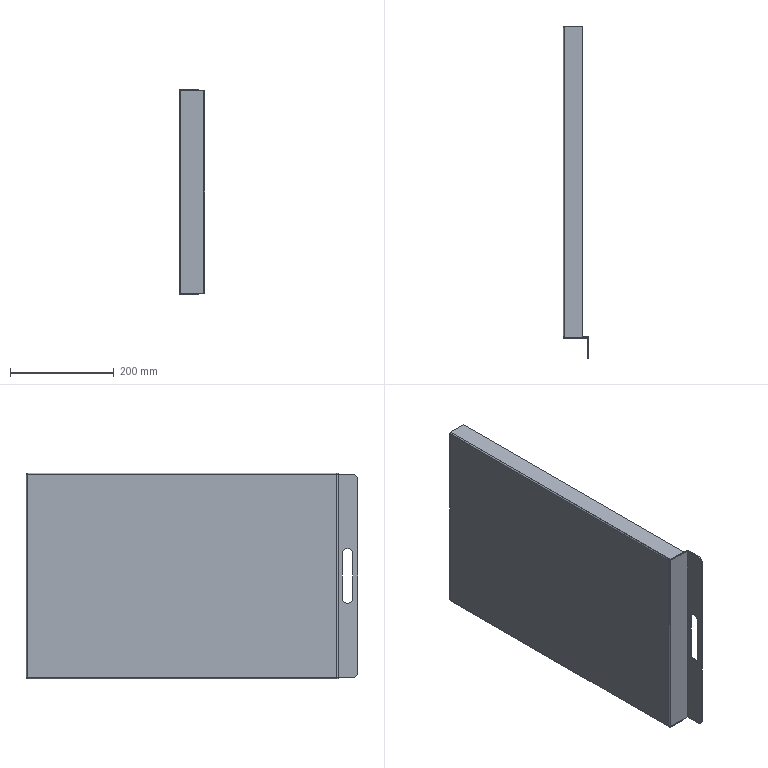Part | STEP file | HJDX-306 | 1 solid | 49 faces | box 50 x 638 x 396 mm | volume 649767 mm3 | plane 34 | cylinder 15 | commonest cylinder face diameters 1 x5 5 x5 20 x5
STEP:
#1=CARTESIAN_POINT('',(46.,-318.,-52.752));
#2=VERTEX_POINT('',#1);
#3=CARTESIAN_POINT('',(46.,-308.,-42.752));
#4=VERTEX_POINT('',#3);
#5=CARTESIAN_POINT('',(46.,-318.,-42.752));
#6=DIRECTION('',(1.,0.,0.));
#7=DIRECTION('',(0.,0.,-1.));
#8=AXIS2_PLACEMENT_3D('',#5,#6,#7);
#9=CIRCLE('',#8,10.);
#10=EDGE_CURVE('',#2,#4,#9,.T.);
#11=ORIENTED_EDGE('',*,*,#10,.F.);
#12=CARTESIAN_POINT('',(48.,-318.,-52.752));
#13=VERTEX_POINT('',#12);
#14=CARTESIAN_POINT('',(-2.,-318.,-52.752));
#15=DIRECTION('',(1.,0.,0.));
#16=VECTOR('',#15,1000.);
#17=LINE('',#14,#16);
#18=EDGE_CURVE('',#2,#13,#17,.T.);
#19=ORIENTED_EDGE('',*,*,#18,.T.);
#20=CARTESIAN_POINT('',(48.,-308.,-42.752));
#21=VERTEX_POINT('',#20);
#22=CARTESIAN_POINT('',(48.,-318.,-42.752));
#23=DIRECTION('',(-1.,0.,0.));
#24=DIRECTION('',(0.,0.,-1.));
#25=AXIS2_PLACEMENT_3D('',#22,#23,#24);
#26=CIRCLE('',#25,10.);
#27=EDGE_CURVE('',#21,#13,#26,.T.);
#28=ORIENTED_EDGE('',*,*,#27,.F.);
#29=CARTESIAN_POINT('',(-2.,-308.,-42.752));
#30=DIRECTION('',(-1.,0.,0.));
#31=VECTOR('',#30,1000.);
#32=LINE('',#29,#31);
#33=EDGE_CURVE('',#21,#4,#32,.T.);
#34=ORIENTED_EDGE('',*,*,#33,.T.);
#35=EDGE_LOOP('',(#11,#19,#28,#34));
#36=FACE_OUTER_BOUND('',#35,.T.);
#37=CARTESIAN_POINT('',(-2.,-318.,-42.752));
#38=DIRECTION('',(1.,0.,0.));
#39=DIRECTION('',(0.,0.,-1.));
#40=AXIS2_PLACEMENT_3D('',#37,#38,#39);
#41=CYLINDRICAL_SURFACE('',#40,10.);
#42=ADVANCED_FACE('',(#36),#41,.F.);
#43=CARTESIAN_POINT('',(-2.,-297.5,195.5));
#44=VERTEX_POINT('',#43);
#45=CARTESIAN_POINT('',(-2.,297.5,195.5));
#46=VERTEX_POINT('',#45);
#47=CARTESIAN_POINT('',(-2.,0.,195.5));
#48=DIRECTION('',(0.,1.,0.));
#49=VECTOR('',#48,1000.);
#50=LINE('',#47,#49);
#51=EDGE_CURVE('',#44,#46,#50,.T.);
#52=ORIENTED_EDGE('',*,*,#51,.T.);
#53=CARTESIAN_POINT('',(-2.,297.5,-195.5));
#54=VERTEX_POINT('',#53);
#55=CARTESIAN_POINT('',(-2.,297.5,0.));
#56=DIRECTION('',(0.,0.,-1.));
#57=VECTOR('',#56,1000.);
#58=LINE('',#55,#57);
#59=EDGE_CURVE('',#46,#54,#58,.T.);
#60=ORIENTED_EDGE('',*,*,#59,.T.);
#61=CARTESIAN_POINT('',(-2.,-297.5,-195.5));
#62=VERTEX_POINT('',#61);
#63=CARTESIAN_POINT('',(-2.,0.,-195.5));
#64=DIRECTION('',(0.,-1.,0.));
#65=VECTOR('',#64,1000.);
#66=LINE('',#63,#65);
#67=EDGE_CURVE('',#54,#62,#66,.T.);
#68=ORIENTED_EDGE('',*,*,#67,.T.);
#69=CARTESIAN_POINT('',(-2.,-297.5,0.));
#70=DIRECTION('',(0.,0.,1.));
#71=VECTOR('',#70,1000.);
#72=LINE('',#69,#71);
#73=EDGE_CURVE('',#62,#44,#72,.T.);
#74=ORIENTED_EDGE('',*,*,#73,.T.);
#75=EDGE_LOOP('',(#52,#60,#68,#74));
#76=FACE_OUTER_BOUND('',#75,.T.);
#77=CARTESIAN_POINT('',(-2.,0.,0.));
#78=DIRECTION('',(-1.,0.,0.));
#79=DIRECTION('',(0.,0.,1.));
#80=AXIS2_PLACEMENT_3D('',#77,#78,#79);
#81=PLANE('',#80);
#82=ADVANCED_FACE('',(#76),#81,.T.);
#83=CARTESIAN_POINT('',(0.5,300.,195.5));
#84=VERTEX_POINT('',#83);
#85=CARTESIAN_POINT('',(0.5,300.,-195.5));
#86=VERTEX_POINT('',#85);
#87=CARTESIAN_POINT('',(0.5,300.,195.5));
#88=DIRECTION('',(0.,0.,-1.));
#89=VECTOR('',#88,1000.);
#90=LINE('',#87,#89);
#91=EDGE_CURVE('',#84,#86,#90,.T.);
#92=ORIENTED_EDGE('',*,*,#91,.T.);
#93=CARTESIAN_POINT('',(0.5,297.5,-195.5));
#94=DIRECTION('',(0.,0.,1.));
#95=DIRECTION('',(1.,0.,0.));
#96=AXIS2_PLACEMENT_3D('',#93,#94,#95);
#97=CIRCLE('',#96,2.5);
#98=EDGE_CURVE('',#86,#54,#97,.T.);
#99=ORIENTED_EDGE('',*,*,#98,.T.);
#100=ORIENTED_EDGE('',*,*,#59,.F.);
#101=CARTESIAN_POINT('',(0.5,297.5,195.5));
#102=DIRECTION('',(0.,0.,-1.));
#103=DIRECTION('',(1.,0.,0.));
#104=AXIS2_PLACEMENT_3D('',#101,#102,#103);
#105=CIRCLE('',#104,2.5);
#106=EDGE_CURVE('',#46,#84,#105,.T.);
#107=ORIENTED_EDGE('',*,*,#106,.T.);
#108=EDGE_LOOP('',(#92,#99,#100,#107));
#109=FACE_OUTER_BOUND('',#108,.T.);
#110=CARTESIAN_POINT('',(0.5,297.5,195.5));
#111=DIRECTION('',(0.,0.,1.));
#112=DIRECTION('',(1.,0.,0.));
#113=AXIS2_PLACEMENT_3D('',#110,#111,#112);
#114=CYLINDRICAL_SURFACE('',#113,2.5);
#115=ADVANCED_FACE('',(#109),#114,.T.);
#116=CARTESIAN_POINT('',(0.5,-297.5,198.));
#117=VERTEX_POINT('',#116);
#118=CARTESIAN_POINT('',(0.5,297.5,198.));
#119=VERTEX_POINT('',#118);
#120=CARTESIAN_POINT('',(0.5,-300.,198.));
#121=DIRECTION('',(0.,1.,0.));
#122=VECTOR('',#121,1000.);
#123=LINE('',#120,#122);
#124=EDGE_CURVE('',#117,#119,#123,.T.);
#125=ORIENTED_EDGE('',*,*,#124,.T.);
#126=CARTESIAN_POINT('',(0.5,297.5,195.5));
#127=DIRECTION('',(0.,-1.,0.));
#128=DIRECTION('',(0.,0.,-1.));
#129=AXIS2_PLACEMENT_3D('',#126,#127,#128);
#130=CIRCLE('',#129,2.5);
#131=EDGE_CURVE('',#119,#46,#130,.T.);
#132=ORIENTED_EDGE('',*,*,#131,.T.);
#133=ORIENTED_EDGE('',*,*,#51,.F.);
#134=CARTESIAN_POINT('',(0.5,-297.5,195.5));
#135=DIRECTION('',(0.,1.,0.));
#136=DIRECTION('',(0.,0.,-1.));
#137=AXIS2_PLACEMENT_3D('',#134,#135,#136);
#138=CIRCLE('',#137,2.5);
#139=EDGE_CURVE('',#44,#117,#138,.T.);
#140=ORIENTED_EDGE('',*,*,#139,.T.);
#141=EDGE_LOOP('',(#125,#132,#133,#140));
#142=FACE_OUTER_BOUND('',#141,.T.);
#143=CARTESIAN_POINT('',(0.5,-300.,195.5));
#144=DIRECTION('',(0.,-1.,0.));
#145=DIRECTION('',(0.,0.,-1.));
#146=AXIS2_PLACEMENT_3D('',#143,#144,#145);
#147=CYLINDRICAL_SURFACE('',#146,2.5);
#148=ADVANCED_FACE('',(#142),#147,.T.);
#149=CARTESIAN_POINT('',(0.5,-300.,-195.5));
#150=VERTEX_POINT('',#149);
#151=CARTESIAN_POINT('',(0.5,-300.,195.5));
#152=VERTEX_POINT('',#151);
#153=CARTESIAN_POINT('',(0.5,-300.,-195.5));
#154=DIRECTION('',(0.,0.,1.));
#155=VECTOR('',#154,1000.);
#156=LINE('',#153,#155);
#157=EDGE_CURVE('',#150,#152,#156,.T.);
#158=ORIENTED_EDGE('',*,*,#157,.T.);
#159=CARTESIAN_POINT('',(0.5,-297.5,195.5));
#160=DIRECTION('',(0.,0.,-1.));
#161=DIRECTION('',(-1.,0.,0.));
#162=AXIS2_PLACEMENT_3D('',#159,#160,#161);
#163=CIRCLE('',#162,2.5);
#164=EDGE_CURVE('',#152,#44,#163,.T.);
#165=ORIENTED_EDGE('',*,*,#164,.T.);
#166=ORIENTED_EDGE('',*,*,#73,.F.);
#167=CARTESIAN_POINT('',(0.5,-297.5,-195.5));
#168=DIRECTION('',(0.,0.,1.));
#169=DIRECTION('',(-1.,0.,0.));
#170=AXIS2_PLACEMENT_3D('',#167,#168,#169);
#171=CIRCLE('',#170,2.5);
#172=EDGE_CURVE('',#62,#150,#171,.T.);
#173=ORIENTED_EDGE('',*,*,#172,.T.);
#174=EDGE_LOOP('',(#158,#165,#166,#173));
#175=FACE_OUTER_BOUND('',#174,.T.);
#176=CARTESIAN_POINT('',(0.5,-297.5,-195.5));
#177=DIRECTION('',(0.,0.,-1.));
#178=DIRECTION('',(-1.,0.,0.));
#179=AXIS2_PLACEMENT_3D('',#176,#177,#178);
#180=CYLINDRICAL_SURFACE('',#179,2.5);
#181=ADVANCED_FACE('',(#175),#180,.T.);
#182=ORIENTED_EDGE('',*,*,#67,.F.);
#183=CARTESIAN_POINT('',(0.5,297.5,-198.));
#184=VERTEX_POINT('',#183);
#185=CARTESIAN_POINT('',(0.5,297.5,-195.5));
#186=DIRECTION('',(0.,-1.,0.));
#187=DIRECTION('',(0.,0.,1.));
#188=AXIS2_PLACEMENT_3D('',#185,#186,#187);
#189=CIRCLE('',#188,2.5);
#190=EDGE_CURVE('',#54,#184,#189,.T.);
#191=ORIENTED_EDGE('',*,*,#190,.T.);
#192=CARTESIAN_POINT('',(0.5,-297.5,-198.));
#193=VERTEX_POINT('',#192);
#194=CARTESIAN_POINT('',(0.5,300.,-198.));
#195=DIRECTION('',(0.,-1.,0.));
#196=VECTOR('',#195,1000.);
#197=LINE('',#194,#196);
#198=EDGE_CURVE('',#184,#193,#197,.T.);
#199=ORIENTED_EDGE('',*,*,#198,.T.);
#200=CARTESIAN_POINT('',(0.5,-297.5,-195.5));
#201=DIRECTION('',(0.,1.,0.));
#202=DIRECTION('',(0.,0.,1.));
#203=AXIS2_PLACEMENT_3D('',#200,#201,#202);
#204=CIRCLE('',#203,2.5);
#205=EDGE_CURVE('',#193,#62,#204,.T.);
#206=ORIENTED_EDGE('',*,*,#205,.T.);
#207=EDGE_LOOP('',(#182,#191,#199,#206));
#208=FACE_OUTER_BOUND('',#207,.T.);
#209=CARTESIAN_POINT('',(0.5,300.,-195.5));
#210=DIRECTION('',(0.,1.,0.));
#211=DIRECTION('',(0.,0.,1.));
#212=AXIS2_PLACEMENT_3D('',#209,#210,#211);
#213=CYLINDRICAL_SURFACE('',#212,2.5);
#214=ADVANCED_FACE('',(#208),#213,.T.);
#215=CARTESIAN_POINT('',(0.,297.5,-195.5));
#216=VERTEX_POINT('',#215);
#217=CARTESIAN_POINT('',(0.5,297.5,-195.5));
#218=DIRECTION('',(-1.,0.,0.));
#219=VECTOR('',#218,1000.);
#220=LINE('',#217,#219);
#221=EDGE_CURVE('',#216,#54,#220,.T.);
#222=ORIENTED_EDGE('',*,*,#221,.T.);
#223=ORIENTED_EDGE('',*,*,#98,.F.);
#224=CARTESIAN_POINT('',(36.,300.,-195.5));
#225=VERTEX_POINT('',#224);
#226=CARTESIAN_POINT('',(0.,300.,-195.5));
#227=DIRECTION('',(1.,0.,0.));
#228=VECTOR('',#227,1000.);
#229=LINE('',#226,#228);
#230=EDGE_CURVE('',#86,#225,#229,.T.);
#231=ORIENTED_EDGE('',*,*,#230,.T.);
#232=CARTESIAN_POINT('',(36.,298.,-195.5));
#233=VERTEX_POINT('',#232);
#234=CARTESIAN_POINT('',(36.,300.,-195.5));
#235=DIRECTION('',(0.,1.,0.));
#236=VECTOR('',#235,1000.);
#237=LINE('',#234,#236);
#238=EDGE_CURVE('',#233,#225,#237,.T.);
#239=ORIENTED_EDGE('',*,*,#238,.F.);
#240=CARTESIAN_POINT('',(0.5,298.,-195.5));
#241=VERTEX_POINT('',#240);
#242=CARTESIAN_POINT('',(0.,298.,-195.5));
#243=DIRECTION('',(1.,0.,0.));
#244=VECTOR('',#243,1000.);
#245=LINE('',#242,#244);
#246=EDGE_CURVE('',#241,#233,#245,.T.);
#247=ORIENTED_EDGE('',*,*,#246,.F.);
#248=CARTESIAN_POINT('',(0.5,297.5,-195.5));
#249=DIRECTION('',(0.,0.,1.));
#250=DIRECTION('',(1.,0.,0.));
#251=AXIS2_PLACEMENT_3D('',#248,#249,#250);
#252=CIRCLE('',#251,0.5);
#253=EDGE_CURVE('',#241,#216,#252,.T.);
#254=ORIENTED_EDGE('',*,*,#253,.T.);
#255=EDGE_LOOP('',(#222,#223,#231,#239,#247,#254));
#256=FACE_OUTER_BOUND('',#255,.T.);
#257=CARTESIAN_POINT('',(0.5,297.5,-195.5));
#258=DIRECTION('',(0.,0.,-1.));
#259=DIRECTION('',(-1.,0.,0.));
#260=AXIS2_PLACEMENT_3D('',#257,#258,#259);
#261=PLANE('',#260);
#262=ADVANCED_FACE('',(#256),#261,.T.);
#263=CARTESIAN_POINT('',(36.,300.,195.5));
#264=VERTEX_POINT('',#263);
#265=CARTESIAN_POINT('',(0.,300.,195.5));
#266=DIRECTION('',(-1.,0.,0.));
#267=VECTOR('',#266,1000.);
#268=LINE('',#265,#267);
#269=EDGE_CURVE('',#264,#84,#268,.T.);
#270=ORIENTED_EDGE('',*,*,#269,.F.);
#271=CARTESIAN_POINT('',(36.,300.,0.));
#272=DIRECTION('',(0.,0.,1.));
#273=VECTOR('',#272,1000.);
#274=LINE('',#271,#273);
#275=EDGE_CURVE('',#225,#264,#274,.T.);
#276=ORIENTED_EDGE('',*,*,#275,.F.);
#277=ORIENTED_EDGE('',*,*,#230,.F.);
#278=ORIENTED_EDGE('',*,*,#91,.F.);
#279=EDGE_LOOP('',(#270,#276,#277,#278));
#280=FACE_OUTER_BOUND('',#279,.T.);
#281=CARTESIAN_POINT('',(0.,300.,0.));
#282=DIRECTION('',(0.,-1.,0.));
#283=DIRECTION('',(1.,0.,0.));
#284=AXIS2_PLACEMENT_3D('',#281,#282,#283);
#285=PLANE('',#284);
#286=ADVANCED_FACE('',(#280),#285,.F.);
#287=CARTESIAN_POINT('',(0.,297.5,195.5));
#288=VERTEX_POINT('',#287);
#289=CARTESIAN_POINT('',(0.5,298.,195.5));
#290=VERTEX_POINT('',#289);
#291=CARTESIAN_POINT('',(0.5,297.5,195.5));
#292=DIRECTION('',(0.,0.,-1.));
#293=DIRECTION('',(1.,0.,0.));
#294=AXIS2_PLACEMENT_3D('',#291,#292,#293);
#295=CIRCLE('',#294,0.5);
#296=EDGE_CURVE('',#288,#290,#295,.T.);
#297=ORIENTED_EDGE('',*,*,#296,.T.);
#298=CARTESIAN_POINT('',(36.,298.,195.5));
#299=VERTEX_POINT('',#298);
#300=CARTESIAN_POINT('',(36.,298.,195.5));
#301=DIRECTION('',(-1.,0.,0.));
#302=VECTOR('',#301,1000.);
#303=LINE('',#300,#302);
#304=EDGE_CURVE('',#299,#290,#303,.T.);
#305=ORIENTED_EDGE('',*,*,#304,.F.);
#306=CARTESIAN_POINT('',(36.,300.,195.5));
#307=DIRECTION('',(0.,-1.,0.));
#308=VECTOR('',#307,1000.);
#309=LINE('',#306,#308);
#310=EDGE_CURVE('',#264,#299,#309,.T.);
#311=ORIENTED_EDGE('',*,*,#310,.F.);
#312=ORIENTED_EDGE('',*,*,#269,.T.);
#313=ORIENTED_EDGE('',*,*,#106,.F.);
#314=CARTESIAN_POINT('',(0.5,297.5,195.5));
#315=DIRECTION('',(-1.,0.,0.));
#316=VECTOR('',#315,1000.);
#317=LINE('',#314,#316);
#318=EDGE_CURVE('',#288,#46,#317,.T.);
#319=ORIENTED_EDGE('',*,*,#318,.F.);
#320=EDGE_LOOP('',(#297,#305,#311,#312,#313,#319));
#321=FACE_OUTER_BOUND('',#320,.T.);
#322=CARTESIAN_POINT('',(0.5,297.5,195.5));
#323=DIRECTION('',(0.,0.,-1.));
#324=DIRECTION('',(-1.,0.,0.));
#325=AXIS2_PLACEMENT_3D('',#322,#323,#324);
#326=PLANE('',#325);
#327=ADVANCED_FACE('',(#321),#326,.F.);
#328=CARTESIAN_POINT('',(0.5,297.5,196.));
#329=VERTEX_POINT('',#328);
#330=CARTESIAN_POINT('',(0.5,297.5,195.5));
#331=DIRECTION('',(0.,-1.,0.));
#332=DIRECTION('',(0.,0.,-1.));
#333=AXIS2_PLACEMENT_3D('',#330,#331,#332);
#334=CIRCLE('',#333,0.5);
#335=EDGE_CURVE('',#329,#288,#334,.T.);
#336=ORIENTED_EDGE('',*,*,#335,.T.);
#337=ORIENTED_EDGE('',*,*,#318,.T.);
#338=ORIENTED_EDGE('',*,*,#131,.F.);
#339=CARTESIAN_POINT('',(0.5,297.5,195.5));
#340=DIRECTION('',(0.,0.,-1.));
#341=VECTOR('',#340,1000.);
#342=LINE('',#339,#341);
#343=EDGE_CURVE('',#119,#329,#342,.T.);
#344=ORIENTED_EDGE('',*,*,#343,.T.);
#345=EDGE_LOOP('',(#336,#337,#338,#344));
#346=FACE_OUTER_BOUND('',#345,.T.);
#347=CARTESIAN_POINT('',(0.5,297.5,195.5));
#348=DIRECTION('',(0.,1.,0.));
#349=DIRECTION('',(0.,0.,1.));
#350=AXIS2_PLACEMENT_3D('',#347,#348,#349);
#351=PLANE('',#350);
#352=ADVANCED_FACE('',(#346),#351,.T.);
#353=CARTESIAN_POINT('',(36.,-300.,198.));
#354=VERTEX_POINT('',#353);
#355=CARTESIAN_POINT('',(0.5,-300.,198.));
#356=VERTEX_POINT('',#355);
#357=CARTESIAN_POINT('',(0.,-300.,198.));
#358=DIRECTION('',(-1.,0.,0.));
#359=VECTOR('',#358,1000.);
#360=LINE('',#357,#359);
#361=EDGE_CURVE('',#354,#356,#360,.T.);
#362=ORIENTED_EDGE('',*,*,#361,.F.);
#363=CARTESIAN_POINT('',(36.,300.,198.));
#364=VERTEX_POINT('',#363);
#365=CARTESIAN_POINT('',(36.,0.,198.));
#366=DIRECTION('',(0.,-1.,0.));
#367=VECTOR('',#366,1000.);
#368=LINE('',#365,#367);
#369=EDGE_CURVE('',#364,#354,#368,.T.);
#370=ORIENTED_EDGE('',*,*,#369,.F.);
#371=CARTESIAN_POINT('',(0.5,300.,198.));
#372=VERTEX_POINT('',#371);
#373=CARTESIAN_POINT('',(0.,300.,198.));
#374=DIRECTION('',(1.,0.,0.));
#375=VECTOR('',#374,1000.);
#376=LINE('',#373,#375);
#377=EDGE_CURVE('',#372,#364,#376,.T.);
#378=ORIENTED_EDGE('',*,*,#377,.F.);
#379=CARTESIAN_POINT('',(0.5,0.,198.));
#380=DIRECTION('',(0.,1.,0.));
#381=VECTOR('',#380,1000.);
#382=LINE('',#379,#381);
#383=EDGE_CURVE('',#119,#372,#382,.T.);
#384=ORIENTED_EDGE('',*,*,#383,.F.);
#385=ORIENTED_EDGE('',*,*,#124,.F.);
#386=CARTESIAN_POINT('',(0.5,0.,198.));
#387=DIRECTION('',(0.,1.,0.));
#388=VECTOR('',#387,1000.);
#389=LINE('',#386,#388);
#390=EDGE_CURVE('',#356,#117,#389,.T.);
#391=ORIENTED_EDGE('',*,*,#390,.F.);
#392=EDGE_LOOP('',(#362,#370,#378,#384,#385,#391));
#393=FACE_OUTER_BOUND('',#392,.T.);
#394=CARTESIAN_POINT('',(0.,0.,198.));
#395=DIRECTION('',(0.,0.,-1.));
#396=DIRECTION('',(-1.,0.,0.));
#397=AXIS2_PLACEMENT_3D('',#394,#395,#396);
#398=PLANE('',#397);
#399=ADVANCED_FACE('',(#393),#398,.F.);
#400=ORIENTED_EDGE('',*,*,#139,.F.);
#401=CARTESIAN_POINT('',(0.,-297.5,195.5));
#402=VERTEX_POINT('',#401);
#403=CARTESIAN_POINT('',(0.5,-297.5,195.5));
#404=DIRECTION('',(1.,0.,0.));
#405=VECTOR('',#404,1000.);
#406=LINE('',#403,#405);
#407=EDGE_CURVE('',#44,#402,#406,.T.);
#408=ORIENTED_EDGE('',*,*,#407,.T.);
#409=CARTESIAN_POINT('',(0.5,-297.5,196.));
#410=VERTEX_POINT('',#409);
#411=CARTESIAN_POINT('',(0.5,-297.5,195.5));
#412=DIRECTION('',(0.,1.,0.));
#413=DIRECTION('',(0.,0.,-1.));
#414=AXIS2_PLACEMENT_3D('',#411,#412,#413);
#415=CIRCLE('',#414,0.5);
#416=EDGE_CURVE('',#402,#410,#415,.T.);
#417=ORIENTED_EDGE('',*,*,#416,.T.);
#418=CARTESIAN_POINT('',(0.5,-297.5,195.5));
#419=DIRECTION('',(0.,0.,1.));
#420=VECTOR('',#419,1000.);
#421=LINE('',#418,#420);
#422=EDGE_CURVE('',#410,#117,#421,.T.);
#423=ORIENTED_EDGE('',*,*,#422,.T.);
#424=EDGE_LOOP('',(#400,#408,#417,#423));
#425=FACE_OUTER_BOUND('',#424,.T.);
#426=CARTESIAN_POINT('',(0.5,-297.5,195.5));
#427=DIRECTION('',(0.,-1.,0.));
#428=DIRECTION('',(0.,0.,-1.));
#429=AXIS2_PLACEMENT_3D('',#426,#427,#428);
#430=PLANE('',#429);
#431=ADVANCED_FACE('',(#425),#430,.T.);
#432=ORIENTED_EDGE('',*,*,#407,.F.);
#433=ORIENTED_EDGE('',*,*,#164,.F.);
#434=CARTESIAN_POINT('',(45.5,-300.,195.5));
#435=VERTEX_POINT('',#434);
#436=CARTESIAN_POINT('',(0.,-300.,195.5));
#437=DIRECTION('',(1.,0.,0.));
#438=VECTOR('',#437,1000.);
#439=LINE('',#436,#438);
#440=EDGE_CURVE('',#152,#435,#439,.T.);
#441=ORIENTED_EDGE('',*,*,#440,.T.);
#442=CARTESIAN_POINT('',(46.,-300.5,195.5));
#443=VERTEX_POINT('',#442);
#444=CARTESIAN_POINT('',(45.5,-300.5,195.5));
#445=DIRECTION('',(0.,0.,-1.));
#446=DIRECTION('',(1.,0.,0.));
#447=AXIS2_PLACEMENT_3D('',#444,#445,#446);
#448=CIRCLE('',#447,0.5);
#449=EDGE_CURVE('',#435,#443,#448,.T.);
#450=ORIENTED_EDGE('',*,*,#449,.T.);
#451=CARTESIAN_POINT('',(46.,-328.,195.5));
#452=VERTEX_POINT('',#451);
#453=CARTESIAN_POINT('',(46.,0.,195.5));
#454=DIRECTION('',(0.,1.,0.));
#455=VECTOR('',#454,1000.);
#456=LINE('',#453,#455);
#457=EDGE_CURVE('',#452,#443,#456,.T.);
#458=ORIENTED_EDGE('',*,*,#457,.F.);
#459=CARTESIAN_POINT('',(48.,-328.,195.5));
#460=VERTEX_POINT('',#459);
#461=CARTESIAN_POINT('',(48.,-328.,195.5));
#462=DIRECTION('',(-1.,0.,0.));
#463=VECTOR('',#462,1000.);
#464=LINE('',#461,#463);
#465=EDGE_CURVE('',#460,#452,#464,.T.);
#466=ORIENTED_EDGE('',*,*,#465,.F.);
#467=CARTESIAN_POINT('',(48.,-300.5,195.5));
#468=VERTEX_POINT('',#467);
#469=CARTESIAN_POINT('',(48.,-338.,195.5));
#470=DIRECTION('',(0.,-1.,0.));
#471=VECTOR('',#470,1000.);
#472=LINE('',#469,#471);
#473=EDGE_CURVE('',#468,#460,#472,.T.);
#474=ORIENTED_EDGE('',*,*,#473,.F.);
#475=CARTESIAN_POINT('',(45.5,-298.,195.5));
#476=VERTEX_POINT('',#475);
#477=CARTESIAN_POINT('',(45.5,-300.5,195.5));
#478=DIRECTION('',(0.,0.,-1.));
#479=DIRECTION('',(1.,0.,0.));
#480=AXIS2_PLACEMENT_3D('',#477,#478,#479);
#481=CIRCLE('',#480,2.5);
#482=EDGE_CURVE('',#476,#468,#481,.T.);
#483=ORIENTED_EDGE('',*,*,#482,.F.);
#484=CARTESIAN_POINT('',(0.5,-298.,195.5));
#485=VERTEX_POINT('',#484);
#486=CARTESIAN_POINT('',(0.,-298.,195.5));
#487=DIRECTION('',(1.,0.,0.));
#488=VECTOR('',#487,1000.);
#489=LINE('',#486,#488);
#490=EDGE_CURVE('',#485,#476,#489,.T.);
#491=ORIENTED_EDGE('',*,*,#490,.F.);
#492=CARTESIAN_POINT('',(0.5,-297.5,195.5));
#493=DIRECTION('',(0.,0.,-1.));
#494=DIRECTION('',(-1.,0.,0.));
#495=AXIS2_PLACEMENT_3D('',#492,#493,#494);
#496=CIRCLE('',#495,0.5);
#497=EDGE_CURVE('',#485,#402,#496,.T.);
#498=ORIENTED_EDGE('',*,*,#497,.T.);
#499=EDGE_LOOP('',(#432,#433,#441,#450,#458,#466,#474,#483,#491,#498));
#500=FACE_OUTER_BOUND('',#499,.T.);
#501=CARTESIAN_POINT('',(0.5,-297.5,195.5));
#502=DIRECTION('',(0.,0.,1.));
#503=DIRECTION('',(1.,0.,0.));
#504=AXIS2_PLACEMENT_3D('',#501,#502,#503);
#505=PLANE('',#504);
#506=ADVANCED_FACE('',(#500),#505,.T.);
#507=ORIENTED_EDGE('',*,*,#440,.F.);
#508=ORIENTED_EDGE('',*,*,#157,.F.);
#509=CARTESIAN_POINT('',(45.5,-300.,-195.5));
#510=VERTEX_POINT('',#509);
#511=CARTESIAN_POINT('',(0.,-300.,-195.5));
#512=DIRECTION('',(-1.,0.,0.));
#513=VECTOR('',#512,1000.);
#514=LINE('',#511,#513);
#515=EDGE_CURVE('',#510,#150,#514,.T.);
#516=ORIENTED_EDGE('',*,*,#515,.F.);
#517=CARTESIAN_POINT('',(45.5,-300.,0.));
#518=DIRECTION('',(0.,0.,-1.));
#519=VECTOR('',#518,1000.);
#520=LINE('',#517,#519);
#521=EDGE_CURVE('',#435,#510,#520,.T.);
#522=ORIENTED_EDGE('',*,*,#521,.F.);
#523=EDGE_LOOP('',(#507,#508,#516,#522));
#524=FACE_OUTER_BOUND('',#523,.T.);
#525=CARTESIAN_POINT('',(0.,-300.,0.));
#526=DIRECTION('',(0.,1.,0.));
#527=DIRECTION('',(-1.,0.,0.));
#528=AXIS2_PLACEMENT_3D('',#525,#526,#527);
#529=PLANE('',#528);
#530=ADVANCED_FACE('',(#524),#529,.F.);
#531=CARTESIAN_POINT('',(0.,-297.5,-195.5));
#532=VERTEX_POINT('',#531);
#533=CARTESIAN_POINT('',(0.5,-298.,-195.5));
#534=VERTEX_POINT('',#533);
#535=CARTESIAN_POINT('',(0.5,-297.5,-195.5));
#536=DIRECTION('',(0.,0.,1.));
#537=DIRECTION('',(-1.,0.,0.));
#538=AXIS2_PLACEMENT_3D('',#535,#536,#537);
#539=CIRCLE('',#538,0.5);
#540=EDGE_CURVE('',#532,#534,#539,.T.);
#541=ORIENTED_EDGE('',*,*,#540,.T.);
#542=CARTESIAN_POINT('',(45.5,-298.,-195.5));
#543=VERTEX_POINT('',#542);
#544=CARTESIAN_POINT('',(48.,-298.,-195.5));
#545=DIRECTION('',(-1.,0.,0.));
#546=VECTOR('',#545,1000.);
#547=LINE('',#544,#546);
#548=EDGE_CURVE('',#543,#534,#547,.T.);
#549=ORIENTED_EDGE('',*,*,#548,.F.);
#550=CARTESIAN_POINT('',(48.,-300.5,-195.5));
#551=VERTEX_POINT('',#550);
#552=CARTESIAN_POINT('',(45.5,-300.5,-195.5));
#553=DIRECTION('',(0.,0.,-1.));
#554=DIRECTION('',(1.,0.,0.));
#555=AXIS2_PLACEMENT_3D('',#552,#553,#554);
#556=CIRCLE('',#555,2.5);
#557=EDGE_CURVE('',#543,#551,#556,.T.);
#558=ORIENTED_EDGE('',*,*,#557,.T.);
#559=CARTESIAN_POINT('',(48.,-328.,-195.5));
#560=VERTEX_POINT('',#559);
#561=CARTESIAN_POINT('',(48.,-300.,-195.5));
#562=DIRECTION('',(0.,1.,0.));
#563=VECTOR('',#562,1000.);
#564=LINE('',#561,#563);
#565=EDGE_CURVE('',#560,#551,#564,.T.);
#566=ORIENTED_EDGE('',*,*,#565,.F.);
#567=CARTESIAN_POINT('',(46.,-328.,-195.5));
#568=VERTEX_POINT('',#567);
#569=CARTESIAN_POINT('',(48.,-328.,-195.5));
#570=DIRECTION('',(1.,0.,0.));
#571=VECTOR('',#570,1000.);
#572=LINE('',#569,#571);
#573=EDGE_CURVE('',#568,#560,#572,.T.);
#574=ORIENTED_EDGE('',*,*,#573,.F.);
#575=CARTESIAN_POINT('',(46.,-300.5,-195.5));
#576=VERTEX_POINT('',#575);
#577=CARTESIAN_POINT('',(46.,0.,-195.5));
#578=DIRECTION('',(0.,-1.,0.));
#579=VECTOR('',#578,1000.);
#580=LINE('',#577,#579);
#581=EDGE_CURVE('',#576,#568,#580,.T.);
#582=ORIENTED_EDGE('',*,*,#581,.F.);
#583=CARTESIAN_POINT('',(45.5,-300.5,-195.5));
#584=DIRECTION('',(0.,0.,1.));
#585=DIRECTION('',(1.,0.,0.));
#586=AXIS2_PLACEMENT_3D('',#583,#584,#585);
#587=CIRCLE('',#586,0.5);
#588=EDGE_CURVE('',#576,#510,#587,.T.);
#589=ORIENTED_EDGE('',*,*,#588,.T.);
#590=ORIENTED_EDGE('',*,*,#515,.T.);
#591=ORIENTED_EDGE('',*,*,#172,.F.);
#592=CARTESIAN_POINT('',(0.5,-297.5,-195.5));
#593=DIRECTION('',(-1.,0.,0.));
#594=VECTOR('',#593,1000.);
#595=LINE('',#592,#594);
#596=EDGE_CURVE('',#532,#62,#595,.T.);
#597=ORIENTED_EDGE('',*,*,#596,.F.);
#598=EDGE_LOOP('',(#541,#549,#558,#566,#574,#582,#589,#590,#591,#597));
#599=FACE_OUTER_BOUND('',#598,.T.);
#600=CARTESIAN_POINT('',(0.5,-297.5,-195.5));
#601=DIRECTION('',(0.,0.,1.));
#602=DIRECTION('',(1.,0.,0.));
#603=AXIS2_PLACEMENT_3D('',#600,#601,#602);
#604=PLANE('',#603);
#605=ADVANCED_FACE('',(#599),#604,.F.);
#606=ORIENTED_EDGE('',*,*,#190,.F.);
#607=ORIENTED_EDGE('',*,*,#221,.F.);
#608=CARTESIAN_POINT('',(0.5,297.5,-196.));
#609=VERTEX_POINT('',#608);
#610=CARTESIAN_POINT('',(0.5,297.5,-195.5));
#611=DIRECTION('',(0.,-1.,0.));
#612=DIRECTION('',(0.,0.,1.));
#613=AXIS2_PLACEMENT_3D('',#610,#611,#612);
#614=CIRCLE('',#613,0.5);
#615=EDGE_CURVE('',#216,#609,#614,.T.);
#616=ORIENTED_EDGE('',*,*,#615,.T.);
#617=CARTESIAN_POINT('',(0.5,297.5,-195.5));
#618=DIRECTION('',(0.,0.,-1.));
#619=VECTOR('',#618,1000.);
#620=LINE('',#617,#619);
#621=EDGE_CURVE('',#609,#184,#620,.T.);
#622=ORIENTED_EDGE('',*,*,#621,.T.);
#623=EDGE_LOOP('',(#606,#607,#616,#622));
#624=FACE_OUTER_BOUND('',#623,.T.);
#625=CARTESIAN_POINT('',(0.5,297.5,-195.5));
#626=DIRECTION('',(0.,1.,0.));
#627=DIRECTION('',(0.,0.,1.));
#628=AXIS2_PLACEMENT_3D('',#625,#626,#627);
#629=PLANE('',#628);
#630=ADVANCED_FACE('',(#624),#629,.T.);
#631=CARTESIAN_POINT('',(0.5,-297.5,-196.));
#632=VERTEX_POINT('',#631);
#633=CARTESIAN_POINT('',(0.5,-297.5,-195.5));
#634=DIRECTION('',(0.,1.,0.));
#635=DIRECTION('',(0.,0.,1.));
#636=AXIS2_PLACEMENT_3D('',#633,#634,#635);
#637=CIRCLE('',#636,0.5);
#638=EDGE_CURVE('',#632,#532,#637,.T.);
#639=ORIENTED_EDGE('',*,*,#638,.T.);
#640=ORIENTED_EDGE('',*,*,#596,.T.);
#641=ORIENTED_EDGE('',*,*,#205,.F.);
#642=CARTESIAN_POINT('',(0.5,-297.5,-195.5));
#643=DIRECTION('',(0.,0.,1.));
#644=VECTOR('',#643,1000.);
#645=LINE('',#642,#644);
#646=EDGE_CURVE('',#193,#632,#645,.T.);
#647=ORIENTED_EDGE('',*,*,#646,.T.);
#648=EDGE_LOOP('',(#639,#640,#641,#647));
#649=FACE_OUTER_BOUND('',#648,.T.);
#650=CARTESIAN_POINT('',(0.5,-297.5,-195.5));
#651=DIRECTION('',(0.,-1.,0.));
#652=DIRECTION('',(0.,0.,-1.));
#653=AXIS2_PLACEMENT_3D('',#650,#651,#652);
#654=PLANE('',#653);
#655=ADVANCED_FACE('',(#649),#654,.T.);
#656=CARTESIAN_POINT('',(36.,300.,-198.));
#657=VERTEX_POINT('',#656);
#658=CARTESIAN_POINT('',(0.5,300.,-198.));
#659=VERTEX_POINT('',#658);
#660=CARTESIAN_POINT('',(0.,300.,-198.));
#661=DIRECTION('',(-1.,0.,0.));
#662=VECTOR('',#661,1000.);
#663=LINE('',#660,#662);
#664=EDGE_CURVE('',#657,#659,#663,.T.);
#665=ORIENTED_EDGE('',*,*,#664,.F.);
#666=CARTESIAN_POINT('',(36.,-300.,-198.));
#667=VERTEX_POINT('',#666);
#668=CARTESIAN_POINT('',(36.,0.,-198.));
#669=DIRECTION('',(0.,1.,0.));
#670=VECTOR('',#669,1000.);
#671=LINE('',#668,#670);
#672=EDGE_CURVE('',#667,#657,#671,.T.);
#673=ORIENTED_EDGE('',*,*,#672,.F.);
#674=CARTESIAN_POINT('',(0.5,-300.,-198.));
#675=VERTEX_POINT('',#674);
#676=CARTESIAN_POINT('',(0.,-300.,-198.));
#677=DIRECTION('',(1.,0.,0.));
#678=VECTOR('',#677,1000.);
#679=LINE('',#676,#678);
#680=EDGE_CURVE('',#675,#667,#679,.T.);
#681=ORIENTED_EDGE('',*,*,#680,.F.);
#682=CARTESIAN_POINT('',(0.5,0.,-198.));
#683=DIRECTION('',(0.,-1.,0.));
#684=VECTOR('',#683,1000.);
#685=LINE('',#682,#684);
#686=EDGE_CURVE('',#193,#675,#685,.T.);
#687=ORIENTED_EDGE('',*,*,#686,.F.);
#688=ORIENTED_EDGE('',*,*,#198,.F.);
#689=CARTESIAN_POINT('',(0.5,0.,-198.));
#690=DIRECTION('',(0.,-1.,0.));
#691=VECTOR('',#690,1000.);
#692=LINE('',#689,#691);
#693=EDGE_CURVE('',#659,#184,#692,.T.);
#694=ORIENTED_EDGE('',*,*,#693,.F.);
#695=EDGE_LOOP('',(#665,#673,#681,#687,#688,#694));
#696=FACE_OUTER_BOUND('',#695,.T.);
#697=CARTESIAN_POINT('',(0.,0.,-198.));
#698=DIRECTION('',(0.,0.,1.));
#699=DIRECTION('',(1.,0.,0.));
#700=AXIS2_PLACEMENT_3D('',#697,#698,#699);
#701=PLANE('',#700);
#702=ADVANCED_FACE('',(#696),#701,.F.);
#703=ORIENTED_EDGE('',*,*,#238,.T.);
#704=ORIENTED_EDGE('',*,*,#275,.T.);
#705=ORIENTED_EDGE('',*,*,#310,.T.);
#706=CARTESIAN_POINT('',(36.,298.,-195.5));
#707=DIRECTION('',(0.,0.,1.));
#708=VECTOR('',#707,1000.);
#709=LINE('',#706,#708);
#710=EDGE_CURVE('',#233,#299,#709,.T.);
#711=ORIENTED_EDGE('',*,*,#710,.F.);
#712=EDGE_LOOP('',(#703,#704,#705,#711));
#713=FACE_OUTER_BOUND('',#712,.T.);
#714=CARTESIAN_POINT('',(36.,300.,-195.5));
#715=DIRECTION('',(-1.,0.,0.));
#716=DIRECTION('',(0.,-1.,0.));
#717=AXIS2_PLACEMENT_3D('',#714,#715,#716);
#718=PLANE('',#717);
#719=ADVANCED_FACE('',(#713),#718,.F.);
#720=CARTESIAN_POINT('',(0.5,300.,196.));
#721=VERTEX_POINT('',#720);
#722=CARTESIAN_POINT('',(0.5,300.,0.));
#723=DIRECTION('',(0.,0.,-1.));
#724=VECTOR('',#723,1000.);
#725=LINE('',#722,#724);
#726=EDGE_CURVE('',#372,#721,#725,.T.);
#727=ORIENTED_EDGE('',*,*,#726,.T.);
#728=CARTESIAN_POINT('',(0.5,0.,196.));
#729=DIRECTION('',(0.,-1.,0.));
#730=VECTOR('',#729,1000.);
#731=LINE('',#728,#730);
#732=EDGE_CURVE('',#721,#329,#731,.T.);
#733=ORIENTED_EDGE('',*,*,#732,.T.);
#734=ORIENTED_EDGE('',*,*,#343,.F.);
#735=ORIENTED_EDGE('',*,*,#383,.T.);
#736=EDGE_LOOP('',(#727,#733,#734,#735));
#737=FACE_OUTER_BOUND('',#736,.T.);
#738=CARTESIAN_POINT('',(0.5,0.,0.));
#739=DIRECTION('',(-1.,0.,0.));
#740=DIRECTION('',(0.,-1.,0.));
#741=AXIS2_PLACEMENT_3D('',#738,#739,#740);
#742=PLANE('',#741);
#743=ADVANCED_FACE('',(#737),#742,.T.);
#744=CARTESIAN_POINT('',(0.5,-300.,196.));
#745=VERTEX_POINT('',#744);
#746=CARTESIAN_POINT('',(0.5,0.,196.));
#747=DIRECTION('',(0.,1.,0.));
#748=VECTOR('',#747,1000.);
#749=LINE('',#746,#748);
#750=EDGE_CURVE('',#745,#410,#749,.T.);
#751=ORIENTED_EDGE('',*,*,#750,.F.);
#752=CARTESIAN_POINT('',(0.5,-300.,0.));
#753=DIRECTION('',(0.,0.,-1.));
#754=VECTOR('',#753,1000.);
#755=LINE('',#752,#754);
#756=EDGE_CURVE('',#356,#745,#755,.T.);
#757=ORIENTED_EDGE('',*,*,#756,.F.);
#758=ORIENTED_EDGE('',*,*,#390,.T.);
#759=ORIENTED_EDGE('',*,*,#422,.F.);
#760=EDGE_LOOP('',(#751,#757,#758,#759));
#761=FACE_OUTER_BOUND('',#760,.T.);
#762=CARTESIAN_POINT('',(0.5,0.,0.));
#763=DIRECTION('',(1.,0.,0.));
#764=DIRECTION('',(0.,1.,0.));
#765=AXIS2_PLACEMENT_3D('',#762,#763,#764);
#766=PLANE('',#765);
#767=ADVANCED_FACE('',(#761),#766,.F.);
#768=CARTESIAN_POINT('',(36.,-300.,196.));
#769=VERTEX_POINT('',#768);
#770=CARTESIAN_POINT('',(36.,-300.,196.));
#771=DIRECTION('',(-1.,0.,0.));
#772=VECTOR('',#771,1000.);
#773=LINE('',#770,#772);
#774=EDGE_CURVE('',#769,#745,#773,.T.);
#775=ORIENTED_EDGE('',*,*,#774,.F.);
#776=CARTESIAN_POINT('',(36.,-300.,198.));
#777=DIRECTION('',(0.,0.,-1.));
#778=VECTOR('',#777,1000.);
#779=LINE('',#776,#778);
#780=EDGE_CURVE('',#354,#769,#779,.T.);
#781=ORIENTED_EDGE('',*,*,#780,.F.);
#782=ORIENTED_EDGE('',*,*,#361,.T.);
#783=ORIENTED_EDGE('',*,*,#756,.T.);
#784=EDGE_LOOP('',(#775,#781,#782,#783));
#785=FACE_OUTER_BOUND('',#784,.T.);
#786=CARTESIAN_POINT('',(36.,-300.,198.));
#787=DIRECTION('',(0.,1.,0.));
#788=DIRECTION('',(0.,0.,1.));
#789=AXIS2_PLACEMENT_3D('',#786,#787,#788);
#790=PLANE('',#789);
#791=ADVANCED_FACE('',(#785),#790,.F.);
#792=CARTESIAN_POINT('',(36.,300.,196.));
#793=VERTEX_POINT('',#792);
#794=CARTESIAN_POINT('',(36.,300.,198.));
#795=DIRECTION('',(0.,0.,-1.));
#796=VECTOR('',#795,1000.);
#797=LINE('',#794,#796);
#798=EDGE_CURVE('',#364,#793,#797,.T.);
#799=ORIENTED_EDGE('',*,*,#798,.F.);
#800=ORIENTED_EDGE('',*,*,#369,.T.);
#801=ORIENTED_EDGE('',*,*,#780,.T.);
#802=CARTESIAN_POINT('',(36.,300.,196.));
#803=DIRECTION('',(0.,-1.,0.));
#804=VECTOR('',#803,1000.);
#805=LINE('',#802,#804);
#806=EDGE_CURVE('',#793,#769,#805,.T.);
#807=ORIENTED_EDGE('',*,*,#806,.F.);
#808=EDGE_LOOP('',(#799,#800,#801,#807));
#809=FACE_OUTER_BOUND('',#808,.T.);
#810=CARTESIAN_POINT('',(36.,300.,198.));
#811=DIRECTION('',(-1.,0.,0.));
#812=DIRECTION('',(0.,0.,1.));
#813=AXIS2_PLACEMENT_3D('',#810,#811,#812);
#814=PLANE('',#813);
#815=ADVANCED_FACE('',(#809),#814,.F.);
#816=ORIENTED_EDGE('',*,*,#377,.T.);
#817=ORIENTED_EDGE('',*,*,#798,.T.);
#818=CARTESIAN_POINT('',(0.,300.,196.));
#819=DIRECTION('',(1.,0.,0.));
#820=VECTOR('',#819,1000.);
#821=LINE('',#818,#820);
#822=EDGE_CURVE('',#721,#793,#821,.T.);
#823=ORIENTED_EDGE('',*,*,#822,.F.);
#824=ORIENTED_EDGE('',*,*,#726,.F.);
#825=EDGE_LOOP('',(#816,#817,#823,#824));
#826=FACE_OUTER_BOUND('',#825,.T.);
#827=CARTESIAN_POINT('',(0.,300.,198.));
#828=DIRECTION('',(0.,-1.,0.));
#829=DIRECTION('',(0.,0.,-1.));
#830=AXIS2_PLACEMENT_3D('',#827,#828,#829);
#831=PLANE('',#830);
#832=ADVANCED_FACE('',(#826),#831,.F.);
#833=ORIENTED_EDGE('',*,*,#588,.F.);
#834=CARTESIAN_POINT('',(46.,-300.5,195.5));
#835=DIRECTION('',(0.,0.,-1.));
#836=VECTOR('',#835,1000.);
#837=LINE('',#834,#836);
#838=EDGE_CURVE('',#443,#576,#837,.T.);
#839=ORIENTED_EDGE('',*,*,#838,.F.);
#840=ORIENTED_EDGE('',*,*,#449,.F.);
#841=ORIENTED_EDGE('',*,*,#521,.T.);
#842=EDGE_LOOP('',(#833,#839,#840,#841));
#843=FACE_OUTER_BOUND('',#842,.T.);
#844=CARTESIAN_POINT('',(45.5,-300.5,195.5));
#845=DIRECTION('',(0.,0.,1.));
#846=DIRECTION('',(1.,0.,0.));
#847=AXIS2_PLACEMENT_3D('',#844,#845,#846);
#848=CYLINDRICAL_SURFACE('',#847,0.5);
#849=ADVANCED_FACE('',(#843),#848,.F.);
#850=CARTESIAN_POINT('',(0.5,300.,-196.));
#851=VERTEX_POINT('',#850);
#852=CARTESIAN_POINT('',(0.5,0.,-196.));
#853=DIRECTION('',(0.,-1.,0.));
#854=VECTOR('',#853,1000.);
#855=LINE('',#852,#854);
#856=EDGE_CURVE('',#851,#609,#855,.T.);
#857=ORIENTED_EDGE('',*,*,#856,.F.);
#858=CARTESIAN_POINT('',(0.5,300.,0.));
#859=DIRECTION('',(0.,0.,1.));
#860=VECTOR('',#859,1000.);
#861=LINE('',#858,#860);
#862=EDGE_CURVE('',#659,#851,#861,.T.);
#863=ORIENTED_EDGE('',*,*,#862,.F.);
#864=ORIENTED_EDGE('',*,*,#693,.T.);
#865=ORIENTED_EDGE('',*,*,#621,.F.);
#866=EDGE_LOOP('',(#857,#863,#864,#865));
#867=FACE_OUTER_BOUND('',#866,.T.);
#868=CARTESIAN_POINT('',(0.5,0.,0.));
#869=DIRECTION('',(1.,0.,0.));
#870=DIRECTION('',(0.,1.,0.));
#871=AXIS2_PLACEMENT_3D('',#868,#869,#870);
#872=PLANE('',#871);
#873=ADVANCED_FACE('',(#867),#872,.F.);
#874=CARTESIAN_POINT('',(0.5,-300.,-196.));
#875=VERTEX_POINT('',#874);
#876=CARTESIAN_POINT('',(0.5,-300.,0.));
#877=DIRECTION('',(0.,0.,1.));
#878=VECTOR('',#877,1000.);
#879=LINE('',#876,#878);
#880=EDGE_CURVE('',#675,#875,#879,.T.);
#881=ORIENTED_EDGE('',*,*,#880,.T.);
#882=CARTESIAN_POINT('',(0.5,0.,-196.));
#883=DIRECTION('',(0.,1.,0.));
#884=VECTOR('',#883,1000.);
#885=LINE('',#882,#884);
#886=EDGE_CURVE('',#875,#632,#885,.T.);
#887=ORIENTED_EDGE('',*,*,#886,.T.);
#888=ORIENTED_EDGE('',*,*,#646,.F.);
#889=ORIENTED_EDGE('',*,*,#686,.T.);
#890=EDGE_LOOP('',(#881,#887,#888,#889));
#891=FACE_OUTER_BOUND('',#890,.T.);
#892=CARTESIAN_POINT('',(0.5,0.,0.));
#893=DIRECTION('',(-1.,0.,0.));
#894=DIRECTION('',(0.,-1.,0.));
#895=AXIS2_PLACEMENT_3D('',#892,#893,#894);
#896=PLANE('',#895);
#897=ADVANCED_FACE('',(#891),#896,.T.);
#898=CARTESIAN_POINT('',(36.,300.,-196.));
#899=VERTEX_POINT('',#898);
#900=CARTESIAN_POINT('',(36.,300.,-196.));
#901=DIRECTION('',(-1.,0.,0.));
#902=VECTOR('',#901,1000.);
#903=LINE('',#900,#902);
#904=EDGE_CURVE('',#899,#851,#903,.T.);
#905=ORIENTED_EDGE('',*,*,#904,.F.);
#906=CARTESIAN_POINT('',(36.,300.,-198.));
#907=DIRECTION('',(0.,0.,1.));
#908=VECTOR('',#907,1000.);
#909=LINE('',#906,#908);
#910=EDGE_CURVE('',#657,#899,#909,.T.);
#911=ORIENTED_EDGE('',*,*,#910,.F.);
#912=ORIENTED_EDGE('',*,*,#664,.T.);
#913=ORIENTED_EDGE('',*,*,#862,.T.);
#914=EDGE_LOOP('',(#905,#911,#912,#913));
#915=FACE_OUTER_BOUND('',#914,.T.);
#916=CARTESIAN_POINT('',(36.,300.,-198.));
#917=DIRECTION('',(0.,-1.,0.));
#918=DIRECTION('',(0.,0.,-1.));
#919=AXIS2_PLACEMENT_3D('',#916,#917,#918);
#920=PLANE('',#919);
#921=ADVANCED_FACE('',(#915),#920,.F.);
#922=CARTESIAN_POINT('',(36.,-300.,-196.));
#923=VERTEX_POINT('',#922);
#924=CARTESIAN_POINT('',(36.,-300.,-198.));
#925=DIRECTION('',(0.,0.,1.));
#926=VECTOR('',#925,1000.);
#927=LINE('',#924,#926);
#928=EDGE_CURVE('',#667,#923,#927,.T.);
#929=ORIENTED_EDGE('',*,*,#928,.F.);
#930=ORIENTED_EDGE('',*,*,#672,.T.);
#931=ORIENTED_EDGE('',*,*,#910,.T.);
#932=CARTESIAN_POINT('',(36.,-300.,-196.));
#933=DIRECTION('',(0.,1.,0.));
#934=VECTOR('',#933,1000.);
#935=LINE('',#932,#934);
#936=EDGE_CURVE('',#923,#899,#935,.T.);
#937=ORIENTED_EDGE('',*,*,#936,.F.);
#938=EDGE_LOOP('',(#929,#930,#931,#937));
#939=FACE_OUTER_BOUND('',#938,.T.);
#940=CARTESIAN_POINT('',(36.,-300.,-198.));
#941=DIRECTION('',(-1.,0.,0.));
#942=DIRECTION('',(0.,0.,1.));
#943=AXIS2_PLACEMENT_3D('',#940,#941,#942);
#944=PLANE('',#943);
#945=ADVANCED_FACE('',(#939),#944,.F.);
#946=ORIENTED_EDGE('',*,*,#680,.T.);
#947=ORIENTED_EDGE('',*,*,#928,.T.);
#948=CARTESIAN_POINT('',(0.,-300.,-196.));
#949=DIRECTION('',(1.,0.,0.));
#950=VECTOR('',#949,1000.);
#951=LINE('',#948,#950);
#952=EDGE_CURVE('',#875,#923,#951,.T.);
#953=ORIENTED_EDGE('',*,*,#952,.F.);
#954=ORIENTED_EDGE('',*,*,#880,.F.);
#955=EDGE_LOOP('',(#946,#947,#953,#954));
#956=FACE_OUTER_BOUND('',#955,.T.);
#957=CARTESIAN_POINT('',(0.,-300.,-198.));
#958=DIRECTION('',(0.,1.,0.));
#959=DIRECTION('',(0.,0.,1.));
#960=AXIS2_PLACEMENT_3D('',#957,#958,#959);
#961=PLANE('',#960);
#962=ADVANCED_FACE('',(#956),#961,.F.);
#963=ORIENTED_EDGE('',*,*,#246,.T.);
#964=ORIENTED_EDGE('',*,*,#710,.T.);
#965=ORIENTED_EDGE('',*,*,#304,.T.);
#966=CARTESIAN_POINT('',(0.5,298.,0.));
#967=DIRECTION('',(0.,0.,-1.));
#968=VECTOR('',#967,1000.);
#969=LINE('',#966,#968);
#970=EDGE_CURVE('',#290,#241,#969,.T.);
#971=ORIENTED_EDGE('',*,*,#970,.T.);
#972=EDGE_LOOP('',(#963,#964,#965,#971));
#973=FACE_OUTER_BOUND('',#972,.T.);
#974=CARTESIAN_POINT('',(0.,298.,0.));
#975=DIRECTION('',(0.,-1.,0.));
#976=DIRECTION('',(1.,0.,0.));
#977=AXIS2_PLACEMENT_3D('',#974,#975,#976);
#978=PLANE('',#977);
#979=ADVANCED_FACE('',(#973),#978,.T.);
#980=ORIENTED_EDGE('',*,*,#822,.T.);
#981=ORIENTED_EDGE('',*,*,#806,.T.);
#982=ORIENTED_EDGE('',*,*,#774,.T.);
#983=ORIENTED_EDGE('',*,*,#750,.T.);
#984=CARTESIAN_POINT('',(0.5,0.,196.));
#985=DIRECTION('',(0.,1.,0.));
#986=VECTOR('',#985,1000.);
#987=LINE('',#984,#986);
#988=EDGE_CURVE('',#410,#329,#987,.T.);
#989=ORIENTED_EDGE('',*,*,#988,.T.);
#990=ORIENTED_EDGE('',*,*,#732,.F.);
#991=EDGE_LOOP('',(#980,#981,#982,#983,#989,#990));
#992=FACE_OUTER_BOUND('',#991,.T.);
#993=CARTESIAN_POINT('',(0.,0.,196.));
#994=DIRECTION('',(0.,0.,-1.));
#995=DIRECTION('',(-1.,0.,0.));
#996=AXIS2_PLACEMENT_3D('',#993,#994,#995);
#997=PLANE('',#996);
#998=ADVANCED_FACE('',(#992),#997,.T.);
#999=ORIENTED_EDGE('',*,*,#548,.T.);
#1000=CARTESIAN_POINT('',(0.5,-298.,0.));
#1001=DIRECTION('',(0.,0.,1.));
#1002=VECTOR('',#1001,1000.);
#1003=LINE('',#1000,#1002);
#1004=EDGE_CURVE('',#534,#485,#1003,.T.);
#1005=ORIENTED_EDGE('',*,*,#1004,.T.);
#1006=ORIENTED_EDGE('',*,*,#490,.T.);
#1007=CARTESIAN_POINT('',(45.5,-298.,0.));
#1008=DIRECTION('',(0.,0.,-1.));
#1009=VECTOR('',#1008,1000.);
#1010=LINE('',#1007,#1009);
#1011=EDGE_CURVE('',#476,#543,#1010,.T.);
#1012=ORIENTED_EDGE('',*,*,#1011,.T.);
#1013=EDGE_LOOP('',(#999,#1005,#1006,#1012));
#1014=FACE_OUTER_BOUND('',#1013,.T.);
#1015=CARTESIAN_POINT('',(0.,-298.,0.));
#1016=DIRECTION('',(0.,1.,0.));
#1017=DIRECTION('',(-1.,0.,0.));
#1018=AXIS2_PLACEMENT_3D('',#1015,#1016,#1017);
#1019=PLANE('',#1018);
#1020=ADVANCED_FACE('',(#1014),#1019,.T.);
#1021=ORIENTED_EDGE('',*,*,#457,.T.);
#1022=ORIENTED_EDGE('',*,*,#838,.T.);
#1023=ORIENTED_EDGE('',*,*,#581,.T.);
#1024=CARTESIAN_POINT('',(46.,-338.,-185.5));
#1025=VERTEX_POINT('',#1024);
#1026=CARTESIAN_POINT('',(46.,-328.,-185.5));
#1027=DIRECTION('',(-1.,0.,0.));
#1028=DIRECTION('',(0.,0.,1.));
#1029=AXIS2_PLACEMENT_3D('',#1026,#1027,#1028);
#1030=CIRCLE('',#1029,10.);
#1031=EDGE_CURVE('',#568,#1025,#1030,.T.);
#1032=ORIENTED_EDGE('',*,*,#1031,.T.);
#1033=CARTESIAN_POINT('',(46.,-338.,185.5));
#1034=VERTEX_POINT('',#1033);
#1035=CARTESIAN_POINT('',(46.,-338.,0.));
#1036=DIRECTION('',(0.,0.,1.));
#1037=VECTOR('',#1036,1000.);
#1038=LINE('',#1035,#1037);
#1039=EDGE_CURVE('',#1025,#1034,#1038,.T.);
#1040=ORIENTED_EDGE('',*,*,#1039,.T.);
#1041=CARTESIAN_POINT('',(46.,-328.,185.5));
#1042=DIRECTION('',(-1.,0.,0.));
#1043=DIRECTION('',(0.,0.,1.));
#1044=AXIS2_PLACEMENT_3D('',#1041,#1042,#1043);
#1045=CIRCLE('',#1044,10.);
#1046=EDGE_CURVE('',#1034,#452,#1045,.T.);
#1047=ORIENTED_EDGE('',*,*,#1046,.T.);
#1048=EDGE_LOOP('',(#1021,#1022,#1023,#1032,#1040,#1047));
#1049=FACE_OUTER_BOUND('',#1048,.T.);
#1050=CARTESIAN_POINT('',(46.,-328.,-42.752));
#1051=VERTEX_POINT('',#1050);
#1052=CARTESIAN_POINT('',(46.,-318.,-42.752));
#1053=DIRECTION('',(1.,0.,0.));
#1054=DIRECTION('',(0.,0.,-1.));
#1055=AXIS2_PLACEMENT_3D('',#1052,#1053,#1054);
#1056=CIRCLE('',#1055,10.);
#1057=EDGE_CURVE('',#1051,#2,#1056,.T.);
#1058=ORIENTED_EDGE('',*,*,#1057,.T.);
#1059=ORIENTED_EDGE('',*,*,#10,.T.);
#1060=CARTESIAN_POINT('',(46.,-308.,42.752));
#1061=VERTEX_POINT('',#1060);
#1062=CARTESIAN_POINT('',(46.,-308.,0.));
#1063=DIRECTION('',(0.,0.,1.));
#1064=VECTOR('',#1063,1000.);
#1065=LINE('',#1062,#1064);
#1066=EDGE_CURVE('',#4,#1061,#1065,.T.);
#1067=ORIENTED_EDGE('',*,*,#1066,.T.);
#1068=CARTESIAN_POINT('',(46.,-328.,42.752));
#1069=VERTEX_POINT('',#1068);
#1070=CARTESIAN_POINT('',(46.,-318.,42.752));
#1071=DIRECTION('',(1.,0.,0.));
#1072=DIRECTION('',(0.,0.,-1.));
#1073=AXIS2_PLACEMENT_3D('',#1070,#1071,#1072);
#1074=CIRCLE('',#1073,10.);
#1075=EDGE_CURVE('',#1061,#1069,#1074,.T.);
#1076=ORIENTED_EDGE('',*,*,#1075,.T.);
#1077=CARTESIAN_POINT('',(46.,-328.,0.));
#1078=DIRECTION('',(0.,0.,-1.));
#1079=VECTOR('',#1078,1000.);
#1080=LINE('',#1077,#1079);
#1081=EDGE_CURVE('',#1069,#1051,#1080,.T.);
#1082=ORIENTED_EDGE('',*,*,#1081,.T.);
#1083=EDGE_LOOP('',(#1058,#1059,#1067,#1076,#1082));
#1084=FACE_BOUND('',#1083,.T.);
#1085=CARTESIAN_POINT('',(46.,0.,0.));
#1086=DIRECTION('',(-1.,0.,0.));
#1087=DIRECTION('',(0.,0.,1.));
#1088=AXIS2_PLACEMENT_3D('',#1085,#1086,#1087);
#1089=PLANE('',#1088);
#1090=ADVANCED_FACE('',(#1049,#1084),#1089,.T.);
#1091=ORIENTED_EDGE('',*,*,#952,.T.);
#1092=ORIENTED_EDGE('',*,*,#936,.T.);
#1093=ORIENTED_EDGE('',*,*,#904,.T.);
#1094=ORIENTED_EDGE('',*,*,#856,.T.);
#1095=CARTESIAN_POINT('',(0.5,0.,-196.));
#1096=DIRECTION('',(0.,-1.,0.));
#1097=VECTOR('',#1096,1000.);
#1098=LINE('',#1095,#1097);
#1099=EDGE_CURVE('',#609,#632,#1098,.T.);
#1100=ORIENTED_EDGE('',*,*,#1099,.T.);
#1101=ORIENTED_EDGE('',*,*,#886,.F.);
#1102=EDGE_LOOP('',(#1091,#1092,#1093,#1094,#1100,#1101));
#1103=FACE_OUTER_BOUND('',#1102,.T.);
#1104=CARTESIAN_POINT('',(0.,0.,-196.));
#1105=DIRECTION('',(0.,0.,1.));
#1106=DIRECTION('',(1.,0.,0.));
#1107=AXIS2_PLACEMENT_3D('',#1104,#1105,#1106);
#1108=PLANE('',#1107);
#1109=ADVANCED_FACE('',(#1103),#1108,.T.);
#1110=ORIENTED_EDGE('',*,*,#253,.F.);
#1111=ORIENTED_EDGE('',*,*,#970,.F.);
#1112=ORIENTED_EDGE('',*,*,#296,.F.);
#1113=CARTESIAN_POINT('',(0.,297.5,195.5));
#1114=DIRECTION('',(0.,0.,1.));
#1115=VECTOR('',#1114,1000.);
#1116=LINE('',#1113,#1115);
#1117=EDGE_CURVE('',#216,#288,#1116,.T.);
#1118=ORIENTED_EDGE('',*,*,#1117,.F.);
#1119=EDGE_LOOP('',(#1110,#1111,#1112,#1118));
#1120=FACE_OUTER_BOUND('',#1119,.T.);
#1121=CARTESIAN_POINT('',(0.5,297.5,195.5));
#1122=DIRECTION('',(0.,0.,1.));
#1123=DIRECTION('',(1.,0.,0.));
#1124=AXIS2_PLACEMENT_3D('',#1121,#1122,#1123);
#1125=CYLINDRICAL_SURFACE('',#1124,0.5);
#1126=ADVANCED_FACE('',(#1120),#1125,.F.);
#1127=CARTESIAN_POINT('',(0.,-300.,195.5));
#1128=DIRECTION('',(0.,-1.,0.));
#1129=VECTOR('',#1128,1000.);
#1130=LINE('',#1127,#1129);
#1131=EDGE_CURVE('',#288,#402,#1130,.T.);
#1132=ORIENTED_EDGE('',*,*,#1131,.F.);
#1133=ORIENTED_EDGE('',*,*,#335,.F.);
#1134=ORIENTED_EDGE('',*,*,#988,.F.);
#1135=ORIENTED_EDGE('',*,*,#416,.F.);
#1136=EDGE_LOOP('',(#1132,#1133,#1134,#1135));
#1137=FACE_OUTER_BOUND('',#1136,.T.);
#1138=CARTESIAN_POINT('',(0.5,-300.,195.5));
#1139=DIRECTION('',(0.,-1.,0.));
#1140=DIRECTION('',(0.,0.,-1.));
#1141=AXIS2_PLACEMENT_3D('',#1138,#1139,#1140);
#1142=CYLINDRICAL_SURFACE('',#1141,0.5);
#1143=ADVANCED_FACE('',(#1137),#1142,.F.);
#1144=CARTESIAN_POINT('',(48.,-300.5,195.5));
#1145=DIRECTION('',(0.,0.,-1.));
#1146=VECTOR('',#1145,1000.);
#1147=LINE('',#1144,#1146);
#1148=EDGE_CURVE('',#468,#551,#1147,.T.);
#1149=ORIENTED_EDGE('',*,*,#1148,.T.);
#1150=ORIENTED_EDGE('',*,*,#557,.F.);
#1151=ORIENTED_EDGE('',*,*,#1011,.F.);
#1152=ORIENTED_EDGE('',*,*,#482,.T.);
#1153=EDGE_LOOP('',(#1149,#1150,#1151,#1152));
#1154=FACE_OUTER_BOUND('',#1153,.T.);
#1155=CARTESIAN_POINT('',(45.5,-300.5,195.5));
#1156=DIRECTION('',(0.,0.,1.));
#1157=DIRECTION('',(1.,0.,0.));
#1158=AXIS2_PLACEMENT_3D('',#1155,#1156,#1157);
#1159=CYLINDRICAL_SURFACE('',#1158,2.5);
#1160=ADVANCED_FACE('',(#1154),#1159,.T.);
#1161=ORIENTED_EDGE('',*,*,#497,.F.);
#1162=ORIENTED_EDGE('',*,*,#1004,.F.);
#1163=ORIENTED_EDGE('',*,*,#540,.F.);
#1164=CARTESIAN_POINT('',(0.,-297.5,-195.5));
#1165=DIRECTION('',(0.,0.,-1.));
#1166=VECTOR('',#1165,1000.);
#1167=LINE('',#1164,#1166);
#1168=EDGE_CURVE('',#402,#532,#1167,.T.);
#1169=ORIENTED_EDGE('',*,*,#1168,.F.);
#1170=EDGE_LOOP('',(#1161,#1162,#1163,#1169));
#1171=FACE_OUTER_BOUND('',#1170,.T.);
#1172=CARTESIAN_POINT('',(0.5,-297.5,-195.5));
#1173=DIRECTION('',(0.,0.,-1.));
#1174=DIRECTION('',(-1.,0.,0.));
#1175=AXIS2_PLACEMENT_3D('',#1172,#1173,#1174);
#1176=CYLINDRICAL_SURFACE('',#1175,0.5);
#1177=ADVANCED_FACE('',(#1171),#1176,.F.);
#1178=ORIENTED_EDGE('',*,*,#1046,.F.);
#1179=CARTESIAN_POINT('',(48.,-338.,185.5));
#1180=VERTEX_POINT('',#1179);
#1181=CARTESIAN_POINT('',(48.,-338.,185.5));
#1182=DIRECTION('',(1.,0.,0.));
#1183=VECTOR('',#1182,1000.);
#1184=LINE('',#1181,#1183);
#1185=EDGE_CURVE('',#1034,#1180,#1184,.T.);
#1186=ORIENTED_EDGE('',*,*,#1185,.T.);
#1187=CARTESIAN_POINT('',(48.,-328.,185.5));
#1188=DIRECTION('',(-1.,0.,0.));
#1189=DIRECTION('',(0.,0.,1.));
#1190=AXIS2_PLACEMENT_3D('',#1187,#1188,#1189);
#1191=CIRCLE('',#1190,10.);
#1192=EDGE_CURVE('',#1180,#460,#1191,.T.);
#1193=ORIENTED_EDGE('',*,*,#1192,.T.);
#1194=ORIENTED_EDGE('',*,*,#465,.T.);
#1195=EDGE_LOOP('',(#1178,#1186,#1193,#1194));
#1196=FACE_OUTER_BOUND('',#1195,.T.);
#1197=CARTESIAN_POINT('',(48.,-328.,185.5));
#1198=DIRECTION('',(-1.,0.,0.));
#1199=DIRECTION('',(0.,0.,1.));
#1200=AXIS2_PLACEMENT_3D('',#1197,#1198,#1199);
#1201=CYLINDRICAL_SURFACE('',#1200,10.);
#1202=ADVANCED_FACE('',(#1196),#1201,.T.);
#1203=CARTESIAN_POINT('',(48.,-338.,-185.5));
#1204=VERTEX_POINT('',#1203);
#1205=CARTESIAN_POINT('',(48.,-338.,-185.5));
#1206=DIRECTION('',(-1.,0.,0.));
#1207=VECTOR('',#1206,1000.);
#1208=LINE('',#1205,#1207);
#1209=EDGE_CURVE('',#1204,#1025,#1208,.T.);
#1210=ORIENTED_EDGE('',*,*,#1209,.F.);
#1211=CARTESIAN_POINT('',(48.,-338.,-195.5));
#1212=DIRECTION('',(0.,0.,-1.));
#1213=VECTOR('',#1212,1000.);
#1214=LINE('',#1211,#1213);
#1215=EDGE_CURVE('',#1180,#1204,#1214,.T.);
#1216=ORIENTED_EDGE('',*,*,#1215,.F.);
#1217=ORIENTED_EDGE('',*,*,#1185,.F.);
#1218=ORIENTED_EDGE('',*,*,#1039,.F.);
#1219=EDGE_LOOP('',(#1210,#1216,#1217,#1218));
#1220=FACE_OUTER_BOUND('',#1219,.T.);
#1221=CARTESIAN_POINT('',(48.,-338.,-195.5));
#1222=DIRECTION('',(0.,1.,0.));
#1223=DIRECTION('',(-1.,0.,0.));
#1224=AXIS2_PLACEMENT_3D('',#1221,#1222,#1223);
#1225=PLANE('',#1224);
#1226=ADVANCED_FACE('',(#1220),#1225,.F.);
#1227=ORIENTED_EDGE('',*,*,#1031,.F.);
#1228=ORIENTED_EDGE('',*,*,#573,.T.);
#1229=CARTESIAN_POINT('',(48.,-328.,-185.5));
#1230=DIRECTION('',(-1.,0.,0.));
#1231=DIRECTION('',(0.,0.,1.));
#1232=AXIS2_PLACEMENT_3D('',#1229,#1230,#1231);
#1233=CIRCLE('',#1232,10.);
#1234=EDGE_CURVE('',#560,#1204,#1233,.T.);
#1235=ORIENTED_EDGE('',*,*,#1234,.T.);
#1236=ORIENTED_EDGE('',*,*,#1209,.T.);
#1237=EDGE_LOOP('',(#1227,#1228,#1235,#1236));
#1238=FACE_OUTER_BOUND('',#1237,.T.);
#1239=CARTESIAN_POINT('',(48.,-328.,-185.5));
#1240=DIRECTION('',(-1.,0.,0.));
#1241=DIRECTION('',(0.,0.,1.));
#1242=AXIS2_PLACEMENT_3D('',#1239,#1240,#1241);
#1243=CYLINDRICAL_SURFACE('',#1242,10.);
#1244=ADVANCED_FACE('',(#1238),#1243,.T.);
#1245=ORIENTED_EDGE('',*,*,#33,.F.);
#1246=CARTESIAN_POINT('',(48.,-308.,42.752));
#1247=VERTEX_POINT('',#1246);
#1248=CARTESIAN_POINT('',(48.,-308.,42.752));
#1249=DIRECTION('',(0.,0.,-1.));
#1250=VECTOR('',#1249,1000.);
#1251=LINE('',#1248,#1250);
#1252=EDGE_CURVE('',#1247,#21,#1251,.T.);
#1253=ORIENTED_EDGE('',*,*,#1252,.F.);
#1254=CARTESIAN_POINT('',(-2.,-308.,42.752));
#1255=DIRECTION('',(1.,0.,0.));
#1256=VECTOR('',#1255,1000.);
#1257=LINE('',#1254,#1256);
#1258=EDGE_CURVE('',#1061,#1247,#1257,.T.);
#1259=ORIENTED_EDGE('',*,*,#1258,.F.);
#1260=ORIENTED_EDGE('',*,*,#1066,.F.);
#1261=EDGE_LOOP('',(#1245,#1253,#1259,#1260));
#1262=FACE_OUTER_BOUND('',#1261,.T.);
#1263=CARTESIAN_POINT('',(-2.,-308.,42.752));
#1264=DIRECTION('',(0.,1.,0.));
#1265=DIRECTION('',(0.,0.,1.));
#1266=AXIS2_PLACEMENT_3D('',#1263,#1264,#1265);
#1267=PLANE('',#1266);
#1268=ADVANCED_FACE('',(#1262),#1267,.F.);
#1269=ORIENTED_EDGE('',*,*,#18,.F.);
#1270=ORIENTED_EDGE('',*,*,#1057,.F.);
#1271=CARTESIAN_POINT('',(48.,-328.,-42.752));
#1272=VERTEX_POINT('',#1271);
#1273=CARTESIAN_POINT('',(-2.,-328.,-42.752));
#1274=DIRECTION('',(-1.,0.,0.));
#1275=VECTOR('',#1274,1000.);
#1276=LINE('',#1273,#1275);
#1277=EDGE_CURVE('',#1272,#1051,#1276,.T.);
#1278=ORIENTED_EDGE('',*,*,#1277,.F.);
#1279=CARTESIAN_POINT('',(48.,-318.,-42.752));
#1280=DIRECTION('',(-1.,0.,0.));
#1281=DIRECTION('',(0.,0.,-1.));
#1282=AXIS2_PLACEMENT_3D('',#1279,#1280,#1281);
#1283=CIRCLE('',#1282,10.);
#1284=EDGE_CURVE('',#13,#1272,#1283,.T.);
#1285=ORIENTED_EDGE('',*,*,#1284,.F.);
#1286=EDGE_LOOP('',(#1269,#1270,#1278,#1285));
#1287=FACE_OUTER_BOUND('',#1286,.T.);
#1288=CARTESIAN_POINT('',(-2.,-318.,-42.752));
#1289=DIRECTION('',(1.,0.,0.));
#1290=DIRECTION('',(0.,0.,-1.));
#1291=AXIS2_PLACEMENT_3D('',#1288,#1289,#1290);
#1292=CYLINDRICAL_SURFACE('',#1291,10.);
#1293=ADVANCED_FACE('',(#1287),#1292,.F.);
#1294=CARTESIAN_POINT('',(48.,-328.,42.752));
#1295=VERTEX_POINT('',#1294);
#1296=CARTESIAN_POINT('',(-2.,-328.,42.752));
#1297=DIRECTION('',(-1.,0.,0.));
#1298=VECTOR('',#1297,1000.);
#1299=LINE('',#1296,#1298);
#1300=EDGE_CURVE('',#1295,#1069,#1299,.T.);
#1301=ORIENTED_EDGE('',*,*,#1300,.F.);
#1302=CARTESIAN_POINT('',(48.,-328.,42.752));
#1303=DIRECTION('',(0.,0.,1.));
#1304=VECTOR('',#1303,1000.);
#1305=LINE('',#1302,#1304);
#1306=EDGE_CURVE('',#1272,#1295,#1305,.T.);
#1307=ORIENTED_EDGE('',*,*,#1306,.F.);
#1308=ORIENTED_EDGE('',*,*,#1277,.T.);
#1309=ORIENTED_EDGE('',*,*,#1081,.F.);
#1310=EDGE_LOOP('',(#1301,#1307,#1308,#1309));
#1311=FACE_OUTER_BOUND('',#1310,.T.);
#1312=CARTESIAN_POINT('',(-2.,-328.,42.752));
#1313=DIRECTION('',(0.,-1.,0.));
#1314=DIRECTION('',(0.,0.,-1.));
#1315=AXIS2_PLACEMENT_3D('',#1312,#1313,#1314);
#1316=PLANE('',#1315);
#1317=ADVANCED_FACE('',(#1311),#1316,.F.);
#1318=ORIENTED_EDGE('',*,*,#1258,.T.);
#1319=CARTESIAN_POINT('',(48.,-318.,42.752));
#1320=DIRECTION('',(-1.,0.,0.));
#1321=DIRECTION('',(0.,0.,-1.));
#1322=AXIS2_PLACEMENT_3D('',#1319,#1320,#1321);
#1323=CIRCLE('',#1322,10.);
#1324=EDGE_CURVE('',#1295,#1247,#1323,.T.);
#1325=ORIENTED_EDGE('',*,*,#1324,.F.);
#1326=ORIENTED_EDGE('',*,*,#1300,.T.);
#1327=ORIENTED_EDGE('',*,*,#1075,.F.);
#1328=EDGE_LOOP('',(#1318,#1325,#1326,#1327));
#1329=FACE_OUTER_BOUND('',#1328,.T.);
#1330=CARTESIAN_POINT('',(-2.,-318.,42.752));
#1331=DIRECTION('',(1.,0.,0.));
#1332=DIRECTION('',(0.,0.,-1.));
#1333=AXIS2_PLACEMENT_3D('',#1330,#1331,#1332);
#1334=CYLINDRICAL_SURFACE('',#1333,10.);
#1335=ADVANCED_FACE('',(#1329),#1334,.F.);
#1336=ORIENTED_EDGE('',*,*,#1099,.F.);
#1337=ORIENTED_EDGE('',*,*,#615,.F.);
#1338=CARTESIAN_POINT('',(0.,300.,-195.5));
#1339=DIRECTION('',(0.,1.,0.));
#1340=VECTOR('',#1339,1000.);
#1341=LINE('',#1338,#1340);
#1342=EDGE_CURVE('',#532,#216,#1341,.T.);
#1343=ORIENTED_EDGE('',*,*,#1342,.F.);
#1344=ORIENTED_EDGE('',*,*,#638,.F.);
#1345=EDGE_LOOP('',(#1336,#1337,#1343,#1344));
#1346=FACE_OUTER_BOUND('',#1345,.T.);
#1347=CARTESIAN_POINT('',(0.5,300.,-195.5));
#1348=DIRECTION('',(0.,1.,0.));
#1349=DIRECTION('',(0.,0.,1.));
#1350=AXIS2_PLACEMENT_3D('',#1347,#1348,#1349);
#1351=CYLINDRICAL_SURFACE('',#1350,0.5);
#1352=ADVANCED_FACE('',(#1346),#1351,.F.);
#1353=ORIENTED_EDGE('',*,*,#1342,.T.);
#1354=ORIENTED_EDGE('',*,*,#1117,.T.);
#1355=ORIENTED_EDGE('',*,*,#1131,.T.);
#1356=ORIENTED_EDGE('',*,*,#1168,.T.);
#1357=EDGE_LOOP('',(#1353,#1354,#1355,#1356));
#1358=FACE_OUTER_BOUND('',#1357,.T.);
#1359=CARTESIAN_POINT('',(0.,0.,0.));
#1360=DIRECTION('',(-1.,0.,0.));
#1361=DIRECTION('',(0.,0.,1.));
#1362=AXIS2_PLACEMENT_3D('',#1359,#1360,#1361);
#1363=PLANE('',#1362);
#1364=ADVANCED_FACE('',(#1358),#1363,.F.);
#1365=ORIENTED_EDGE('',*,*,#1234,.F.);
#1366=ORIENTED_EDGE('',*,*,#565,.T.);
#1367=ORIENTED_EDGE('',*,*,#1148,.F.);
#1368=ORIENTED_EDGE('',*,*,#473,.T.);
#1369=ORIENTED_EDGE('',*,*,#1192,.F.);
#1370=ORIENTED_EDGE('',*,*,#1215,.T.);
#1371=EDGE_LOOP('',(#1365,#1366,#1367,#1368,#1369,#1370));
#1372=FACE_OUTER_BOUND('',#1371,.T.);
#1373=ORIENTED_EDGE('',*,*,#1324,.T.);
#1374=ORIENTED_EDGE('',*,*,#1252,.T.);
#1375=ORIENTED_EDGE('',*,*,#27,.T.);
#1376=ORIENTED_EDGE('',*,*,#1284,.T.);
#1377=ORIENTED_EDGE('',*,*,#1306,.T.);
#1378=EDGE_LOOP('',(#1373,#1374,#1375,#1376,#1377));
#1379=FACE_BOUND('',#1378,.T.);
#1380=CARTESIAN_POINT('',(48.,0.,0.));
#1381=DIRECTION('',(-1.,0.,0.));
#1382=DIRECTION('',(0.,0.,1.));
#1383=AXIS2_PLACEMENT_3D('',#1380,#1381,#1382);
#1384=PLANE('',#1383);
#1385=ADVANCED_FACE('',(#1372,#1379),#1384,.F.);
#1386=CLOSED_SHELL('',(#42,#82,#115,#148,#181,#214,#262,#286,#327,#352,#399,#431,#506,#530,#605,#630,#655,#702,#719,#743,#767,#791,#815,#832,#849,#873,#897,#921,#945,#962,#979,#998,#1020,#1090,#1109,#1126,#1143,#1160,#1177,#1202,#1226,#1244,#1268,#1293,#1317,#1335,#1352,#1364,#1385));
#1387=MANIFOLD_SOLID_BREP('',#1386);
#1388=CARTESIAN_POINT('',(0.,0.,0.));
#1389=DIRECTION('',(0.,0.,1.));
#1390=DIRECTION('',(1.,0.,0.));
#1391=AXIS2_PLACEMENT_3D('',#1388,#1389,#1390);
#1392=(LENGTH_UNIT()NAMED_UNIT(*)SI_UNIT(.MILLI.,.METRE.));
#1393=UNCERTAINTY_MEASURE_WITH_UNIT(LENGTH_MEASURE(0.00001),#1392,'','');
#1394=(NAMED_UNIT(*)PLANE_ANGLE_UNIT()SI_UNIT($,.RADIAN.));
#1395=(NAMED_UNIT(*)SI_UNIT($,.STERADIAN.)SOLID_ANGLE_UNIT());
#1396=(GEOMETRIC_REPRESENTATION_CONTEXT(3)GLOBAL_UNCERTAINTY_ASSIGNED_CONTEXT((#1393))GLOBAL_UNIT_ASSIGNED_CONTEXT((#1392,#1394,#1395))REPRESENTATION_CONTEXT('',''));
#1397=ADVANCED_BREP_SHAPE_REPRESENTATION('',(#1387,#1391),#1396);